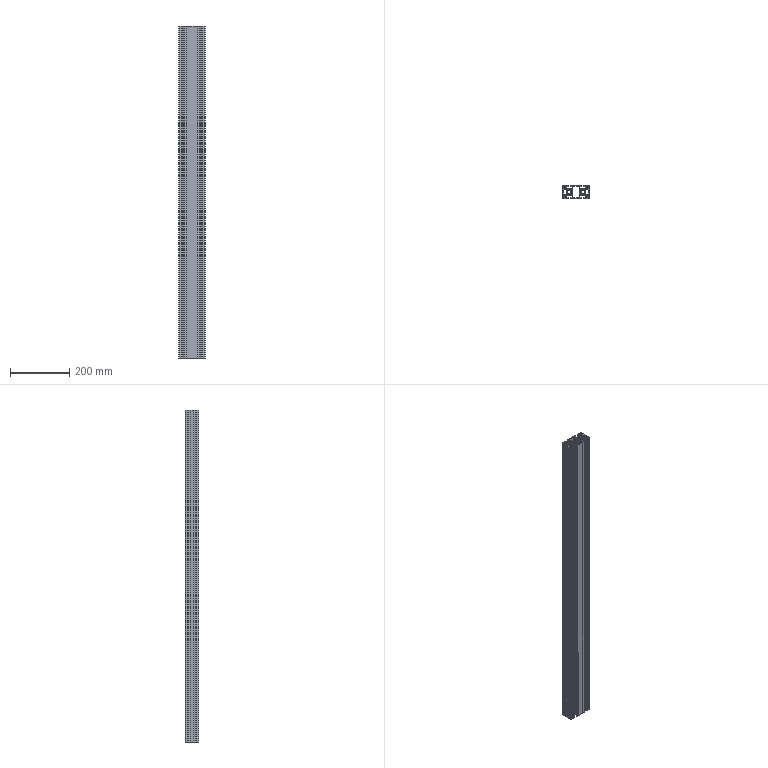Part | STEP file | 4590-1120 aluminium profile (bottom rear cross 2) | 1 solid | 366 faces | box 90 x 45 x 1120 mm | volume 1313429 mm3 | plane 254 | cylinder 112 | commonest cylinder face diameters 2 x64 8 x20 12 x16 4 x12